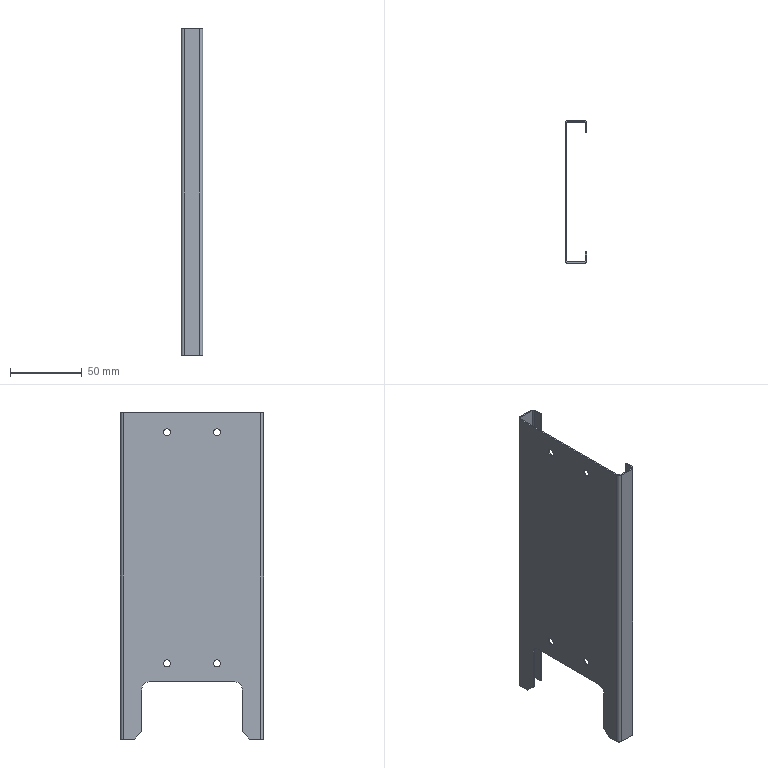Part | SolidWorks | features BaseBody 1 | 1 solid | 54 faces | box 15 x 100 x 228 mm | volume 28896 mm3 | plane 36 | cylinder 18 | commonest cylinder face diameters 5 x8 2 x4 4 x4 10 x2
STEP:
#1=CARTESIAN_POINT('',(0.,90.,-114.));
#2=VERTEX_POINT('',#1);
#3=CARTESIAN_POINT('',(0.,85.,-109.));
#4=VERTEX_POINT('',#3);
#5=CARTESIAN_POINT('',(0.,45.,-69.));
#6=DIRECTION('',(0.,-0.7071,0.7071));
#7=VECTOR('',#6,1000.);
#8=LINE('',#5,#7);
#9=EDGE_CURVE('',#2,#4,#8,.T.);
#10=ORIENTED_EDGE('',*,*,#9,.F.);
#11=CARTESIAN_POINT('',(1.,90.,-114.));
#12=VERTEX_POINT('',#11);
#13=CARTESIAN_POINT('',(0.,90.,-114.));
#14=DIRECTION('',(-1.,0.,0.));
#15=VECTOR('',#14,1000.);
#16=LINE('',#13,#15);
#17=EDGE_CURVE('',#12,#2,#16,.T.);
#18=ORIENTED_EDGE('',*,*,#17,.F.);
#19=CARTESIAN_POINT('',(1.,85.,-109.));
#20=VERTEX_POINT('',#19);
#21=CARTESIAN_POINT('',(1.,85.,-109.));
#22=DIRECTION('',(0.,0.7071,-0.7071));
#23=VECTOR('',#22,1000.);
#24=LINE('',#21,#23);
#25=EDGE_CURVE('',#20,#12,#24,.T.);
#26=ORIENTED_EDGE('',*,*,#25,.F.);
#27=CARTESIAN_POINT('',(1.,85.,-109.));
#28=DIRECTION('',(1.,0.,0.));
#29=VECTOR('',#28,1000.);
#30=LINE('',#27,#29);
#31=EDGE_CURVE('',#4,#20,#30,.T.);
#32=ORIENTED_EDGE('',*,*,#31,.F.);
#33=EDGE_LOOP('',(#10,#18,#26,#32));
#34=FACE_OUTER_BOUND('',#33,.T.);
#35=CARTESIAN_POINT('',(10.,85.,-109.));
#36=DIRECTION('',(0.,-0.7071,-0.7071));
#37=DIRECTION('',(0.,-0.7071,0.7071));
#38=AXIS2_PLACEMENT_3D('',#35,#36,#37);
#39=PLANE('',#38);
#40=ADVANCED_FACE('',(#34),#39,.T.);
#41=CARTESIAN_POINT('',(1.,10.,-114.));
#42=VERTEX_POINT('',#41);
#43=CARTESIAN_POINT('',(1.,15.,-109.));
#44=VERTEX_POINT('',#43);
#45=CARTESIAN_POINT('',(1.,15.,-109.));
#46=DIRECTION('',(0.,0.7071,0.7071));
#47=VECTOR('',#46,1000.);
#48=LINE('',#45,#47);
#49=EDGE_CURVE('',#42,#44,#48,.T.);
#50=ORIENTED_EDGE('',*,*,#49,.F.);
#51=CARTESIAN_POINT('',(0.,10.,-114.));
#52=VERTEX_POINT('',#51);
#53=CARTESIAN_POINT('',(1.,10.,-114.));
#54=DIRECTION('',(1.,0.,0.));
#55=VECTOR('',#54,1000.);
#56=LINE('',#53,#55);
#57=EDGE_CURVE('',#52,#42,#56,.T.);
#58=ORIENTED_EDGE('',*,*,#57,.F.);
#59=CARTESIAN_POINT('',(0.,15.,-109.));
#60=VERTEX_POINT('',#59);
#61=CARTESIAN_POINT('',(0.,5.,-119.));
#62=DIRECTION('',(0.,-0.7071,-0.7071));
#63=VECTOR('',#62,1000.);
#64=LINE('',#61,#63);
#65=EDGE_CURVE('',#60,#52,#64,.T.);
#66=ORIENTED_EDGE('',*,*,#65,.F.);
#67=CARTESIAN_POINT('',(0.,15.,-109.));
#68=DIRECTION('',(-1.,0.,0.));
#69=VECTOR('',#68,1000.);
#70=LINE('',#67,#69);
#71=EDGE_CURVE('',#44,#60,#70,.T.);
#72=ORIENTED_EDGE('',*,*,#71,.F.);
#73=EDGE_LOOP('',(#50,#58,#66,#72));
#74=FACE_OUTER_BOUND('',#73,.T.);
#75=CARTESIAN_POINT('',(10.,15.,-109.));
#76=DIRECTION('',(0.,0.7071,-0.7071));
#77=DIRECTION('',(-1.,0.,0.));
#78=AXIS2_PLACEMENT_3D('',#75,#76,#77);
#79=PLANE('',#78);
#80=ADVANCED_FACE('',(#74),#79,.T.);
#81=CARTESIAN_POINT('',(1.,80.,-74.));
#82=VERTEX_POINT('',#81);
#83=CARTESIAN_POINT('',(1.,85.,-79.));
#84=VERTEX_POINT('',#83);
#85=CARTESIAN_POINT('',(1.,80.,-79.));
#86=DIRECTION('',(-1.,0.,0.));
#87=DIRECTION('',(0.,0.,1.));
#88=AXIS2_PLACEMENT_3D('',#85,#86,#87);
#89=CIRCLE('',#88,5.);
#90=EDGE_CURVE('',#82,#84,#89,.T.);
#91=ORIENTED_EDGE('',*,*,#90,.F.);
#92=CARTESIAN_POINT('',(0.,80.,-74.));
#93=VERTEX_POINT('',#92);
#94=CARTESIAN_POINT('',(1.,80.,-74.));
#95=DIRECTION('',(1.,0.,0.));
#96=VECTOR('',#95,1000.);
#97=LINE('',#94,#96);
#98=EDGE_CURVE('',#93,#82,#97,.T.);
#99=ORIENTED_EDGE('',*,*,#98,.F.);
#100=CARTESIAN_POINT('',(0.,85.,-79.));
#101=VERTEX_POINT('',#100);
#102=CARTESIAN_POINT('',(0.,80.,-79.));
#103=DIRECTION('',(1.,0.,0.));
#104=DIRECTION('',(0.,0.,1.));
#105=AXIS2_PLACEMENT_3D('',#102,#103,#104);
#106=CIRCLE('',#105,5.);
#107=EDGE_CURVE('',#101,#93,#106,.T.);
#108=ORIENTED_EDGE('',*,*,#107,.F.);
#109=CARTESIAN_POINT('',(0.,85.,-79.));
#110=DIRECTION('',(-1.,0.,0.));
#111=VECTOR('',#110,1000.);
#112=LINE('',#109,#111);
#113=EDGE_CURVE('',#84,#101,#112,.T.);
#114=ORIENTED_EDGE('',*,*,#113,.F.);
#115=EDGE_LOOP('',(#91,#99,#108,#114));
#116=FACE_OUTER_BOUND('',#115,.T.);
#117=CARTESIAN_POINT('',(10.,80.,-79.));
#118=DIRECTION('',(1.,0.,0.));
#119=DIRECTION('',(0.,0.,-1.));
#120=AXIS2_PLACEMENT_3D('',#117,#118,#119);
#121=CYLINDRICAL_SURFACE('',#120,5.);
#122=ADVANCED_FACE('',(#116),#121,.F.);
#123=CARTESIAN_POINT('',(1.,15.,-79.));
#124=VERTEX_POINT('',#123);
#125=CARTESIAN_POINT('',(1.,20.,-74.));
#126=VERTEX_POINT('',#125);
#127=CARTESIAN_POINT('',(1.,20.,-79.));
#128=DIRECTION('',(-1.,0.,0.));
#129=DIRECTION('',(0.,0.,1.));
#130=AXIS2_PLACEMENT_3D('',#127,#128,#129);
#131=CIRCLE('',#130,5.);
#132=EDGE_CURVE('',#124,#126,#131,.T.);
#133=ORIENTED_EDGE('',*,*,#132,.F.);
#134=CARTESIAN_POINT('',(0.,15.,-79.));
#135=VERTEX_POINT('',#134);
#136=CARTESIAN_POINT('',(1.,15.,-79.));
#137=DIRECTION('',(1.,0.,0.));
#138=VECTOR('',#137,1000.);
#139=LINE('',#136,#138);
#140=EDGE_CURVE('',#135,#124,#139,.T.);
#141=ORIENTED_EDGE('',*,*,#140,.F.);
#142=CARTESIAN_POINT('',(0.,20.,-74.));
#143=VERTEX_POINT('',#142);
#144=CARTESIAN_POINT('',(0.,20.,-79.));
#145=DIRECTION('',(1.,0.,0.));
#146=DIRECTION('',(0.,0.,1.));
#147=AXIS2_PLACEMENT_3D('',#144,#145,#146);
#148=CIRCLE('',#147,5.);
#149=EDGE_CURVE('',#143,#135,#148,.T.);
#150=ORIENTED_EDGE('',*,*,#149,.F.);
#151=CARTESIAN_POINT('',(0.,20.,-74.));
#152=DIRECTION('',(-1.,0.,0.));
#153=VECTOR('',#152,1000.);
#154=LINE('',#151,#153);
#155=EDGE_CURVE('',#126,#143,#154,.T.);
#156=ORIENTED_EDGE('',*,*,#155,.F.);
#157=EDGE_LOOP('',(#133,#141,#150,#156));
#158=FACE_OUTER_BOUND('',#157,.T.);
#159=CARTESIAN_POINT('',(10.,20.,-79.));
#160=DIRECTION('',(1.,0.,0.));
#161=DIRECTION('',(0.,0.,-1.));
#162=AXIS2_PLACEMENT_3D('',#159,#160,#161);
#163=CYLINDRICAL_SURFACE('',#162,5.);
#164=ADVANCED_FACE('',(#158),#163,.F.);
#165=CARTESIAN_POINT('',(1.,67.5,98.));
#166=VERTEX_POINT('',#165);
#167=CARTESIAN_POINT('',(0.,67.5,98.));
#168=VERTEX_POINT('',#167);
#169=CARTESIAN_POINT('',(10.,67.5,98.));
#170=DIRECTION('',(-1.,0.,0.));
#171=VECTOR('',#170,1000.);
#172=LINE('',#169,#171);
#173=EDGE_CURVE('',#166,#168,#172,.T.);
#174=ORIENTED_EDGE('',*,*,#173,.F.);
#175=CARTESIAN_POINT('',(1.,67.5,103.));
#176=VERTEX_POINT('',#175);
#177=CARTESIAN_POINT('',(1.,67.5,100.5));
#178=DIRECTION('',(-1.,0.,0.));
#179=DIRECTION('',(0.,0.,1.));
#180=AXIS2_PLACEMENT_3D('',#177,#178,#179);
#181=CIRCLE('',#180,2.5);
#182=EDGE_CURVE('',#176,#166,#181,.T.);
#183=ORIENTED_EDGE('',*,*,#182,.F.);
#184=CARTESIAN_POINT('',(0.,67.5,103.));
#185=VERTEX_POINT('',#184);
#186=CARTESIAN_POINT('',(10.,67.5,103.));
#187=DIRECTION('',(-1.,0.,0.));
#188=VECTOR('',#187,1000.);
#189=LINE('',#186,#188);
#190=EDGE_CURVE('',#176,#185,#189,.T.);
#191=ORIENTED_EDGE('',*,*,#190,.T.);
#192=CARTESIAN_POINT('',(0.,67.5,100.5));
#193=DIRECTION('',(-1.,0.,0.));
#194=DIRECTION('',(0.,0.,1.));
#195=AXIS2_PLACEMENT_3D('',#192,#193,#194);
#196=CIRCLE('',#195,2.5);
#197=EDGE_CURVE('',#185,#168,#196,.T.);
#198=ORIENTED_EDGE('',*,*,#197,.T.);
#199=EDGE_LOOP('',(#174,#183,#191,#198));
#200=FACE_OUTER_BOUND('',#199,.T.);
#201=CARTESIAN_POINT('',(10.,67.5,100.5));
#202=DIRECTION('',(-1.,0.,0.));
#203=DIRECTION('',(0.,0.,1.));
#204=AXIS2_PLACEMENT_3D('',#201,#202,#203);
#205=CYLINDRICAL_SURFACE('',#204,2.5);
#206=ADVANCED_FACE('',(#200),#205,.F.);
#207=CARTESIAN_POINT('',(1.,32.5,-63.6));
#208=VERTEX_POINT('',#207);
#209=CARTESIAN_POINT('',(0.,32.5,-63.6));
#210=VERTEX_POINT('',#209);
#211=CARTESIAN_POINT('',(10.,32.5,-63.6));
#212=DIRECTION('',(-1.,0.,0.));
#213=VECTOR('',#212,1000.);
#214=LINE('',#211,#213);
#215=EDGE_CURVE('',#208,#210,#214,.T.);
#216=ORIENTED_EDGE('',*,*,#215,.F.);
#217=CARTESIAN_POINT('',(1.,32.5,-58.6));
#218=VERTEX_POINT('',#217);
#219=CARTESIAN_POINT('',(1.,32.5,-61.1));
#220=DIRECTION('',(-1.,0.,0.));
#221=DIRECTION('',(0.,0.,1.));
#222=AXIS2_PLACEMENT_3D('',#219,#220,#221);
#223=CIRCLE('',#222,2.5);
#224=EDGE_CURVE('',#218,#208,#223,.T.);
#225=ORIENTED_EDGE('',*,*,#224,.F.);
#226=CARTESIAN_POINT('',(0.,32.5,-58.6));
#227=VERTEX_POINT('',#226);
#228=CARTESIAN_POINT('',(10.,32.5,-58.6));
#229=DIRECTION('',(-1.,0.,0.));
#230=VECTOR('',#229,1000.);
#231=LINE('',#228,#230);
#232=EDGE_CURVE('',#218,#227,#231,.T.);
#233=ORIENTED_EDGE('',*,*,#232,.T.);
#234=CARTESIAN_POINT('',(0.,32.5,-61.1));
#235=DIRECTION('',(-1.,0.,0.));
#236=DIRECTION('',(0.,0.,1.));
#237=AXIS2_PLACEMENT_3D('',#234,#235,#236);
#238=CIRCLE('',#237,2.5);
#239=EDGE_CURVE('',#227,#210,#238,.T.);
#240=ORIENTED_EDGE('',*,*,#239,.T.);
#241=EDGE_LOOP('',(#216,#225,#233,#240));
#242=FACE_OUTER_BOUND('',#241,.T.);
#243=CARTESIAN_POINT('',(10.,32.5,-61.1));
#244=DIRECTION('',(-1.,0.,0.));
#245=DIRECTION('',(0.,0.,1.));
#246=AXIS2_PLACEMENT_3D('',#243,#244,#245);
#247=CYLINDRICAL_SURFACE('',#246,2.5);
#248=ADVANCED_FACE('',(#242),#247,.F.);
#249=CARTESIAN_POINT('',(1.,67.5,-63.6));
#250=VERTEX_POINT('',#249);
#251=CARTESIAN_POINT('',(0.,67.5,-63.6));
#252=VERTEX_POINT('',#251);
#253=CARTESIAN_POINT('',(10.,67.5,-63.6));
#254=DIRECTION('',(-1.,0.,0.));
#255=VECTOR('',#254,1000.);
#256=LINE('',#253,#255);
#257=EDGE_CURVE('',#250,#252,#256,.T.);
#258=ORIENTED_EDGE('',*,*,#257,.F.);
#259=CARTESIAN_POINT('',(1.,67.5,-58.6));
#260=VERTEX_POINT('',#259);
#261=CARTESIAN_POINT('',(1.,67.5,-61.1));
#262=DIRECTION('',(-1.,0.,0.));
#263=DIRECTION('',(0.,0.,1.));
#264=AXIS2_PLACEMENT_3D('',#261,#262,#263);
#265=CIRCLE('',#264,2.5);
#266=EDGE_CURVE('',#260,#250,#265,.T.);
#267=ORIENTED_EDGE('',*,*,#266,.F.);
#268=CARTESIAN_POINT('',(0.,67.5,-58.6));
#269=VERTEX_POINT('',#268);
#270=CARTESIAN_POINT('',(10.,67.5,-58.6));
#271=DIRECTION('',(-1.,0.,0.));
#272=VECTOR('',#271,1000.);
#273=LINE('',#270,#272);
#274=EDGE_CURVE('',#260,#269,#273,.T.);
#275=ORIENTED_EDGE('',*,*,#274,.T.);
#276=CARTESIAN_POINT('',(0.,67.5,-61.1));
#277=DIRECTION('',(-1.,0.,0.));
#278=DIRECTION('',(0.,0.,1.));
#279=AXIS2_PLACEMENT_3D('',#276,#277,#278);
#280=CIRCLE('',#279,2.5);
#281=EDGE_CURVE('',#269,#252,#280,.T.);
#282=ORIENTED_EDGE('',*,*,#281,.T.);
#283=EDGE_LOOP('',(#258,#267,#275,#282));
#284=FACE_OUTER_BOUND('',#283,.T.);
#285=CARTESIAN_POINT('',(10.,67.5,-61.1));
#286=DIRECTION('',(-1.,0.,0.));
#287=DIRECTION('',(0.,0.,1.));
#288=AXIS2_PLACEMENT_3D('',#285,#286,#287);
#289=CYLINDRICAL_SURFACE('',#288,2.5);
#290=ADVANCED_FACE('',(#284),#289,.F.);
#291=CARTESIAN_POINT('',(0.,85.,-154.));
#292=DIRECTION('',(0.,0.,-1.));
#293=VECTOR('',#292,1000.);
#294=LINE('',#291,#293);
#295=EDGE_CURVE('',#101,#4,#294,.T.);
#296=ORIENTED_EDGE('',*,*,#295,.T.);
#297=ORIENTED_EDGE('',*,*,#31,.T.);
#298=CARTESIAN_POINT('',(1.,85.,-114.));
#299=DIRECTION('',(0.,0.,-1.));
#300=VECTOR('',#299,1000.);
#301=LINE('',#298,#300);
#302=EDGE_CURVE('',#84,#20,#301,.T.);
#303=ORIENTED_EDGE('',*,*,#302,.F.);
#304=ORIENTED_EDGE('',*,*,#113,.T.);
#305=EDGE_LOOP('',(#296,#297,#303,#304));
#306=FACE_OUTER_BOUND('',#305,.T.);
#307=CARTESIAN_POINT('',(10.,85.,-154.));
#308=DIRECTION('',(0.,1.,0.));
#309=DIRECTION('',(1.,0.,0.));
#310=AXIS2_PLACEMENT_3D('',#307,#308,#309);
#311=PLANE('',#310);
#312=ADVANCED_FACE('',(#306),#311,.F.);
#313=CARTESIAN_POINT('',(1.,15.,-114.));
#314=DIRECTION('',(0.,0.,1.));
#315=VECTOR('',#314,1000.);
#316=LINE('',#313,#315);
#317=EDGE_CURVE('',#44,#124,#316,.T.);
#318=ORIENTED_EDGE('',*,*,#317,.F.);
#319=ORIENTED_EDGE('',*,*,#71,.T.);
#320=CARTESIAN_POINT('',(0.,15.,-154.));
#321=DIRECTION('',(0.,0.,1.));
#322=VECTOR('',#321,1000.);
#323=LINE('',#320,#322);
#324=EDGE_CURVE('',#60,#135,#323,.T.);
#325=ORIENTED_EDGE('',*,*,#324,.T.);
#326=ORIENTED_EDGE('',*,*,#140,.T.);
#327=EDGE_LOOP('',(#318,#319,#325,#326));
#328=FACE_OUTER_BOUND('',#327,.T.);
#329=CARTESIAN_POINT('',(10.,15.,-154.));
#330=DIRECTION('',(0.,-1.,0.));
#331=DIRECTION('',(0.,0.,-1.));
#332=AXIS2_PLACEMENT_3D('',#329,#330,#331);
#333=PLANE('',#332);
#334=ADVANCED_FACE('',(#328),#333,.F.);
#335=CARTESIAN_POINT('',(1.,0.,-74.));
#336=DIRECTION('',(0.,1.,0.));
#337=VECTOR('',#336,1000.);
#338=LINE('',#335,#337);
#339=EDGE_CURVE('',#126,#82,#338,.T.);
#340=ORIENTED_EDGE('',*,*,#339,.F.);
#341=ORIENTED_EDGE('',*,*,#155,.T.);
#342=CARTESIAN_POINT('',(0.,15.,-74.));
#343=DIRECTION('',(0.,1.,0.));
#344=VECTOR('',#343,1000.);
#345=LINE('',#342,#344);
#346=EDGE_CURVE('',#143,#93,#345,.T.);
#347=ORIENTED_EDGE('',*,*,#346,.T.);
#348=ORIENTED_EDGE('',*,*,#98,.T.);
#349=EDGE_LOOP('',(#340,#341,#347,#348));
#350=FACE_OUTER_BOUND('',#349,.T.);
#351=CARTESIAN_POINT('',(10.,15.,-74.));
#352=DIRECTION('',(0.,0.,1.));
#353=DIRECTION('',(1.,0.,0.));
#354=AXIS2_PLACEMENT_3D('',#351,#352,#353);
#355=PLANE('',#354);
#356=ADVANCED_FACE('',(#350),#355,.F.);
#357=CARTESIAN_POINT('',(1.,32.5,98.));
#358=VERTEX_POINT('',#357);
#359=CARTESIAN_POINT('',(0.,32.5,98.));
#360=VERTEX_POINT('',#359);
#361=CARTESIAN_POINT('',(10.,32.5,98.));
#362=DIRECTION('',(-1.,0.,0.));
#363=VECTOR('',#362,1000.);
#364=LINE('',#361,#363);
#365=EDGE_CURVE('',#358,#360,#364,.T.);
#366=ORIENTED_EDGE('',*,*,#365,.F.);
#367=CARTESIAN_POINT('',(1.,32.5,103.));
#368=VERTEX_POINT('',#367);
#369=CARTESIAN_POINT('',(1.,32.5,100.5));
#370=DIRECTION('',(-1.,0.,0.));
#371=DIRECTION('',(0.,0.,1.));
#372=AXIS2_PLACEMENT_3D('',#369,#370,#371);
#373=CIRCLE('',#372,2.5);
#374=EDGE_CURVE('',#368,#358,#373,.T.);
#375=ORIENTED_EDGE('',*,*,#374,.F.);
#376=CARTESIAN_POINT('',(0.,32.5,103.));
#377=VERTEX_POINT('',#376);
#378=CARTESIAN_POINT('',(10.,32.5,103.));
#379=DIRECTION('',(-1.,0.,0.));
#380=VECTOR('',#379,1000.);
#381=LINE('',#378,#380);
#382=EDGE_CURVE('',#368,#377,#381,.T.);
#383=ORIENTED_EDGE('',*,*,#382,.T.);
#384=CARTESIAN_POINT('',(0.,32.5,100.5));
#385=DIRECTION('',(-1.,0.,0.));
#386=DIRECTION('',(0.,0.,1.));
#387=AXIS2_PLACEMENT_3D('',#384,#385,#386);
#388=CIRCLE('',#387,2.5);
#389=EDGE_CURVE('',#377,#360,#388,.T.);
#390=ORIENTED_EDGE('',*,*,#389,.T.);
#391=EDGE_LOOP('',(#366,#375,#383,#390));
#392=FACE_OUTER_BOUND('',#391,.T.);
#393=CARTESIAN_POINT('',(10.,32.5,100.5));
#394=DIRECTION('',(-1.,0.,0.));
#395=DIRECTION('',(0.,0.,1.));
#396=AXIS2_PLACEMENT_3D('',#393,#394,#395);
#397=CYLINDRICAL_SURFACE('',#396,2.5);
#398=ADVANCED_FACE('',(#392),#397,.F.);
#399=CARTESIAN_POINT('',(15.,2.,114.));
#400=VERTEX_POINT('',#399);
#401=CARTESIAN_POINT('',(15.,8.,114.));
#402=VERTEX_POINT('',#401);
#403=CARTESIAN_POINT('',(15.,0.,114.));
#404=DIRECTION('',(0.,1.,0.));
#405=VECTOR('',#404,1000.);
#406=LINE('',#403,#405);
#407=EDGE_CURVE('',#400,#402,#406,.T.);
#408=ORIENTED_EDGE('',*,*,#407,.T.);
#409=CARTESIAN_POINT('',(14.,8.,114.));
#410=VERTEX_POINT('',#409);
#411=CARTESIAN_POINT('',(14.,8.,114.));
#412=DIRECTION('',(1.,0.,0.));
#413=VECTOR('',#412,1000.);
#414=LINE('',#411,#413);
#415=EDGE_CURVE('',#410,#402,#414,.T.);
#416=ORIENTED_EDGE('',*,*,#415,.F.);
#417=CARTESIAN_POINT('',(14.,2.,114.));
#418=VERTEX_POINT('',#417);
#419=CARTESIAN_POINT('',(14.,0.,114.));
#420=DIRECTION('',(0.,1.,0.));
#421=VECTOR('',#420,1000.);
#422=LINE('',#419,#421);
#423=EDGE_CURVE('',#418,#410,#422,.T.);
#424=ORIENTED_EDGE('',*,*,#423,.F.);
#425=CARTESIAN_POINT('',(14.,2.,114.));
#426=DIRECTION('',(1.,0.,0.));
#427=VECTOR('',#426,1000.);
#428=LINE('',#425,#427);
#429=EDGE_CURVE('',#418,#400,#428,.T.);
#430=ORIENTED_EDGE('',*,*,#429,.T.);
#431=EDGE_LOOP('',(#408,#416,#424,#430));
#432=FACE_OUTER_BOUND('',#431,.T.);
#433=CARTESIAN_POINT('',(13.,2.,114.));
#434=DIRECTION('',(0.,0.,1.));
#435=DIRECTION('',(1.,0.,0.));
#436=AXIS2_PLACEMENT_3D('',#433,#434,#435);
#437=PLANE('',#436);
#438=ADVANCED_FACE('',(#432),#437,.T.);
#439=CARTESIAN_POINT('',(14.,92.,-114.));
#440=VERTEX_POINT('',#439);
#441=CARTESIAN_POINT('',(14.,98.,-114.));
#442=VERTEX_POINT('',#441);
#443=CARTESIAN_POINT('',(14.,100.,-114.));
#444=DIRECTION('',(0.,1.,0.));
#445=VECTOR('',#444,1000.);
#446=LINE('',#443,#445);
#447=EDGE_CURVE('',#440,#442,#446,.T.);
#448=ORIENTED_EDGE('',*,*,#447,.T.);
#449=CARTESIAN_POINT('',(15.,98.,-114.));
#450=VERTEX_POINT('',#449);
#451=CARTESIAN_POINT('',(14.,98.,-114.));
#452=DIRECTION('',(1.,0.,0.));
#453=VECTOR('',#452,1000.);
#454=LINE('',#451,#453);
#455=EDGE_CURVE('',#442,#450,#454,.T.);
#456=ORIENTED_EDGE('',*,*,#455,.T.);
#457=CARTESIAN_POINT('',(15.,92.,-114.));
#458=VERTEX_POINT('',#457);
#459=CARTESIAN_POINT('',(15.,100.,-114.));
#460=DIRECTION('',(0.,1.,0.));
#461=VECTOR('',#460,1000.);
#462=LINE('',#459,#461);
#463=EDGE_CURVE('',#458,#450,#462,.T.);
#464=ORIENTED_EDGE('',*,*,#463,.F.);
#465=CARTESIAN_POINT('',(15.,92.,-114.));
#466=DIRECTION('',(-1.,0.,0.));
#467=VECTOR('',#466,1000.);
#468=LINE('',#465,#467);
#469=EDGE_CURVE('',#458,#440,#468,.T.);
#470=ORIENTED_EDGE('',*,*,#469,.T.);
#471=EDGE_LOOP('',(#448,#456,#464,#470));
#472=FACE_OUTER_BOUND('',#471,.T.);
#473=CARTESIAN_POINT('',(13.,2.,-114.));
#474=DIRECTION('',(0.,0.,1.));
#475=DIRECTION('',(1.,0.,0.));
#476=AXIS2_PLACEMENT_3D('',#473,#474,#475);
#477=PLANE('',#476);
#478=ADVANCED_FACE('',(#472),#477,.F.);
#479=ORIENTED_EDGE('',*,*,#415,.T.);
#480=CARTESIAN_POINT('',(15.,8.,-114.));
#481=VERTEX_POINT('',#480);
#482=CARTESIAN_POINT('',(15.,8.,-114.));
#483=DIRECTION('',(0.,0.,1.));
#484=VECTOR('',#483,1000.);
#485=LINE('',#482,#484);
#486=EDGE_CURVE('',#481,#402,#485,.T.);
#487=ORIENTED_EDGE('',*,*,#486,.F.);
#488=CARTESIAN_POINT('',(14.,8.,-114.));
#489=VERTEX_POINT('',#488);
#490=CARTESIAN_POINT('',(14.,8.,-114.));
#491=DIRECTION('',(1.,0.,0.));
#492=VECTOR('',#491,1000.);
#493=LINE('',#490,#492);
#494=EDGE_CURVE('',#489,#481,#493,.T.);
#495=ORIENTED_EDGE('',*,*,#494,.F.);
#496=CARTESIAN_POINT('',(14.,8.,-114.));
#497=DIRECTION('',(0.,0.,1.));
#498=VECTOR('',#497,1000.);
#499=LINE('',#496,#498);
#500=EDGE_CURVE('',#489,#410,#499,.T.);
#501=ORIENTED_EDGE('',*,*,#500,.T.);
#502=EDGE_LOOP('',(#479,#487,#495,#501));
#503=FACE_OUTER_BOUND('',#502,.T.);
#504=CARTESIAN_POINT('',(14.,8.,-114.));
#505=DIRECTION('',(0.,-1.,0.));
#506=DIRECTION('',(0.,0.,-1.));
#507=AXIS2_PLACEMENT_3D('',#504,#505,#506);
#508=PLANE('',#507);
#509=ADVANCED_FACE('',(#503),#508,.F.);
#510=ORIENTED_EDGE('',*,*,#423,.T.);
#511=ORIENTED_EDGE('',*,*,#500,.F.);
#512=CARTESIAN_POINT('',(14.,2.,-114.));
#513=VERTEX_POINT('',#512);
#514=CARTESIAN_POINT('',(14.,0.,-114.));
#515=DIRECTION('',(0.,1.,0.));
#516=VECTOR('',#515,1000.);
#517=LINE('',#514,#516);
#518=EDGE_CURVE('',#513,#489,#517,.T.);
#519=ORIENTED_EDGE('',*,*,#518,.F.);
#520=CARTESIAN_POINT('',(14.,2.,-114.));
#521=DIRECTION('',(0.,0.,1.));
#522=VECTOR('',#521,1000.);
#523=LINE('',#520,#522);
#524=EDGE_CURVE('',#513,#418,#523,.T.);
#525=ORIENTED_EDGE('',*,*,#524,.T.);
#526=EDGE_LOOP('',(#510,#511,#519,#525));
#527=FACE_OUTER_BOUND('',#526,.T.);
#528=CARTESIAN_POINT('',(14.,0.,-114.));
#529=DIRECTION('',(1.,0.,0.));
#530=DIRECTION('',(0.,1.,0.));
#531=AXIS2_PLACEMENT_3D('',#528,#529,#530);
#532=PLANE('',#531);
#533=ADVANCED_FACE('',(#527),#532,.F.);
#534=CARTESIAN_POINT('',(13.,1.,114.));
#535=VERTEX_POINT('',#534);
#536=CARTESIAN_POINT('',(13.,2.,114.));
#537=DIRECTION('',(0.,0.,1.));
#538=DIRECTION('',(1.,0.,0.));
#539=AXIS2_PLACEMENT_3D('',#536,#537,#538);
#540=CIRCLE('',#539,1.);
#541=EDGE_CURVE('',#535,#418,#540,.T.);
#542=ORIENTED_EDGE('',*,*,#541,.T.);
#543=ORIENTED_EDGE('',*,*,#524,.F.);
#544=CARTESIAN_POINT('',(13.,1.,-114.));
#545=VERTEX_POINT('',#544);
#546=CARTESIAN_POINT('',(13.,2.,-114.));
#547=DIRECTION('',(0.,0.,1.));
#548=DIRECTION('',(1.,0.,0.));
#549=AXIS2_PLACEMENT_3D('',#546,#547,#548);
#550=CIRCLE('',#549,1.);
#551=EDGE_CURVE('',#545,#513,#550,.T.);
#552=ORIENTED_EDGE('',*,*,#551,.F.);
#553=CARTESIAN_POINT('',(13.,1.,-114.));
#554=DIRECTION('',(0.,0.,1.));
#555=VECTOR('',#554,1000.);
#556=LINE('',#553,#555);
#557=EDGE_CURVE('',#545,#535,#556,.T.);
#558=ORIENTED_EDGE('',*,*,#557,.T.);
#559=EDGE_LOOP('',(#542,#543,#552,#558));
#560=FACE_OUTER_BOUND('',#559,.T.);
#561=CARTESIAN_POINT('',(13.,2.,-114.));
#562=DIRECTION('',(0.,0.,1.));
#563=DIRECTION('',(1.,0.,0.));
#564=AXIS2_PLACEMENT_3D('',#561,#562,#563);
#565=CYLINDRICAL_SURFACE('',#564,1.);
#566=ADVANCED_FACE('',(#560),#565,.F.);
#567=CARTESIAN_POINT('',(2.,1.,114.));
#568=VERTEX_POINT('',#567);
#569=CARTESIAN_POINT('',(0.,1.,114.));
#570=DIRECTION('',(1.,0.,0.));
#571=VECTOR('',#570,1000.);
#572=LINE('',#569,#571);
#573=EDGE_CURVE('',#568,#535,#572,.T.);
#574=ORIENTED_EDGE('',*,*,#573,.T.);
#575=ORIENTED_EDGE('',*,*,#557,.F.);
#576=CARTESIAN_POINT('',(2.,1.,-114.));
#577=VERTEX_POINT('',#576);
#578=CARTESIAN_POINT('',(0.,1.,-114.));
#579=DIRECTION('',(1.,0.,0.));
#580=VECTOR('',#579,1000.);
#581=LINE('',#578,#580);
#582=EDGE_CURVE('',#577,#545,#581,.T.);
#583=ORIENTED_EDGE('',*,*,#582,.F.);
#584=CARTESIAN_POINT('',(2.,1.,-114.));
#585=DIRECTION('',(0.,0.,1.));
#586=VECTOR('',#585,1000.);
#587=LINE('',#584,#586);
#588=EDGE_CURVE('',#577,#568,#587,.T.);
#589=ORIENTED_EDGE('',*,*,#588,.T.);
#590=EDGE_LOOP('',(#574,#575,#583,#589));
#591=FACE_OUTER_BOUND('',#590,.T.);
#592=CARTESIAN_POINT('',(0.,1.,-114.));
#593=DIRECTION('',(0.,-1.,0.));
#594=DIRECTION('',(0.,0.,-1.));
#595=AXIS2_PLACEMENT_3D('',#592,#593,#594);
#596=PLANE('',#595);
#597=ADVANCED_FACE('',(#591),#596,.F.);
#598=CARTESIAN_POINT('',(1.,2.,114.));
#599=VERTEX_POINT('',#598);
#600=CARTESIAN_POINT('',(2.,2.,114.));
#601=DIRECTION('',(0.,0.,1.));
#602=DIRECTION('',(1.,0.,0.));
#603=AXIS2_PLACEMENT_3D('',#600,#601,#602);
#604=CIRCLE('',#603,1.);
#605=EDGE_CURVE('',#599,#568,#604,.T.);
#606=ORIENTED_EDGE('',*,*,#605,.T.);
#607=ORIENTED_EDGE('',*,*,#588,.F.);
#608=CARTESIAN_POINT('',(1.,2.,-114.));
#609=VERTEX_POINT('',#608);
#610=CARTESIAN_POINT('',(2.,2.,-114.));
#611=DIRECTION('',(0.,0.,1.));
#612=DIRECTION('',(1.,0.,0.));
#613=AXIS2_PLACEMENT_3D('',#610,#611,#612);
#614=CIRCLE('',#613,1.);
#615=EDGE_CURVE('',#609,#577,#614,.T.);
#616=ORIENTED_EDGE('',*,*,#615,.F.);
#617=CARTESIAN_POINT('',(1.,2.,-114.));
#618=DIRECTION('',(0.,0.,1.));
#619=VECTOR('',#618,1000.);
#620=LINE('',#617,#619);
#621=EDGE_CURVE('',#609,#599,#620,.T.);
#622=ORIENTED_EDGE('',*,*,#621,.T.);
#623=EDGE_LOOP('',(#606,#607,#616,#622));
#624=FACE_OUTER_BOUND('',#623,.T.);
#625=CARTESIAN_POINT('',(2.,2.,-114.));
#626=DIRECTION('',(0.,0.,1.));
#627=DIRECTION('',(1.,0.,0.));
#628=AXIS2_PLACEMENT_3D('',#625,#626,#627);
#629=CYLINDRICAL_SURFACE('',#628,1.);
#630=ADVANCED_FACE('',(#624),#629,.F.);
#631=ORIENTED_EDGE('',*,*,#374,.T.);
#632=CARTESIAN_POINT('',(1.,32.5,100.5));
#633=DIRECTION('',(-1.,0.,0.));
#634=DIRECTION('',(0.,0.,1.));
#635=AXIS2_PLACEMENT_3D('',#632,#633,#634);
#636=CIRCLE('',#635,2.5);
#637=EDGE_CURVE('',#358,#368,#636,.T.);
#638=ORIENTED_EDGE('',*,*,#637,.T.);
#639=EDGE_LOOP('',(#631,#638));
#640=FACE_BOUND('',#639,.T.);
#641=ORIENTED_EDGE('',*,*,#266,.T.);
#642=CARTESIAN_POINT('',(1.,67.5,-61.1));
#643=DIRECTION('',(-1.,0.,0.));
#644=DIRECTION('',(0.,0.,1.));
#645=AXIS2_PLACEMENT_3D('',#642,#643,#644);
#646=CIRCLE('',#645,2.5);
#647=EDGE_CURVE('',#250,#260,#646,.T.);
#648=ORIENTED_EDGE('',*,*,#647,.T.);
#649=EDGE_LOOP('',(#641,#648));
#650=FACE_BOUND('',#649,.T.);
#651=ORIENTED_EDGE('',*,*,#224,.T.);
#652=CARTESIAN_POINT('',(1.,32.5,-61.1));
#653=DIRECTION('',(-1.,0.,0.));
#654=DIRECTION('',(0.,0.,1.));
#655=AXIS2_PLACEMENT_3D('',#652,#653,#654);
#656=CIRCLE('',#655,2.5);
#657=EDGE_CURVE('',#208,#218,#656,.T.);
#658=ORIENTED_EDGE('',*,*,#657,.T.);
#659=EDGE_LOOP('',(#651,#658));
#660=FACE_BOUND('',#659,.T.);
#661=ORIENTED_EDGE('',*,*,#182,.T.);
#662=CARTESIAN_POINT('',(1.,67.5,100.5));
#663=DIRECTION('',(-1.,0.,0.));
#664=DIRECTION('',(0.,0.,1.));
#665=AXIS2_PLACEMENT_3D('',#662,#663,#664);
#666=CIRCLE('',#665,2.5);
#667=EDGE_CURVE('',#166,#176,#666,.T.);
#668=ORIENTED_EDGE('',*,*,#667,.T.);
#669=EDGE_LOOP('',(#661,#668));
#670=FACE_BOUND('',#669,.T.);
#671=CARTESIAN_POINT('',(1.,0.,-114.));
#672=DIRECTION('',(0.,-1.,0.));
#673=VECTOR('',#672,1000.);
#674=LINE('',#671,#673);
#675=EDGE_CURVE('',#42,#609,#674,.T.);
#676=ORIENTED_EDGE('',*,*,#675,.F.);
#677=ORIENTED_EDGE('',*,*,#49,.T.);
#678=ORIENTED_EDGE('',*,*,#317,.T.);
#679=ORIENTED_EDGE('',*,*,#132,.T.);
#680=ORIENTED_EDGE('',*,*,#339,.T.);
#681=ORIENTED_EDGE('',*,*,#90,.T.);
#682=ORIENTED_EDGE('',*,*,#302,.T.);
#683=ORIENTED_EDGE('',*,*,#25,.T.);
#684=CARTESIAN_POINT('',(1.,98.,-114.));
#685=VERTEX_POINT('',#684);
#686=CARTESIAN_POINT('',(1.,0.,-114.));
#687=DIRECTION('',(0.,-1.,0.));
#688=VECTOR('',#687,1000.);
#689=LINE('',#686,#688);
#690=EDGE_CURVE('',#685,#12,#689,.T.);
#691=ORIENTED_EDGE('',*,*,#690,.F.);
#692=CARTESIAN_POINT('',(1.,98.,114.));
#693=VERTEX_POINT('',#692);
#694=CARTESIAN_POINT('',(1.,98.,-114.));
#695=DIRECTION('',(0.,0.,1.));
#696=VECTOR('',#695,1000.);
#697=LINE('',#694,#696);
#698=EDGE_CURVE('',#685,#693,#697,.T.);
#699=ORIENTED_EDGE('',*,*,#698,.T.);
#700=CARTESIAN_POINT('',(1.,0.,114.));
#701=DIRECTION('',(0.,-1.,0.));
#702=VECTOR('',#701,1000.);
#703=LINE('',#700,#702);
#704=EDGE_CURVE('',#693,#599,#703,.T.);
#705=ORIENTED_EDGE('',*,*,#704,.T.);
#706=ORIENTED_EDGE('',*,*,#621,.F.);
#707=EDGE_LOOP('',(#676,#677,#678,#679,#680,#681,#682,#683,#691,#699,#705,#706));
#708=FACE_OUTER_BOUND('',#707,.T.);
#709=CARTESIAN_POINT('',(1.,0.,-114.));
#710=DIRECTION('',(-1.,0.,0.));
#711=DIRECTION('',(0.,0.,1.));
#712=AXIS2_PLACEMENT_3D('',#709,#710,#711);
#713=PLANE('',#712);
#714=ADVANCED_FACE('',(#640,#650,#660,#670,#708),#713,.F.);
#715=CARTESIAN_POINT('',(2.,99.,114.));
#716=VERTEX_POINT('',#715);
#717=CARTESIAN_POINT('',(2.,98.,114.));
#718=DIRECTION('',(0.,0.,1.));
#719=DIRECTION('',(1.,0.,0.));
#720=AXIS2_PLACEMENT_3D('',#717,#718,#719);
#721=CIRCLE('',#720,1.);
#722=EDGE_CURVE('',#716,#693,#721,.T.);
#723=ORIENTED_EDGE('',*,*,#722,.T.);
#724=ORIENTED_EDGE('',*,*,#698,.F.);
#725=CARTESIAN_POINT('',(2.,99.,-114.));
#726=VERTEX_POINT('',#725);
#727=CARTESIAN_POINT('',(2.,98.,-114.));
#728=DIRECTION('',(0.,0.,1.));
#729=DIRECTION('',(1.,0.,0.));
#730=AXIS2_PLACEMENT_3D('',#727,#728,#729);
#731=CIRCLE('',#730,1.);
#732=EDGE_CURVE('',#726,#685,#731,.T.);
#733=ORIENTED_EDGE('',*,*,#732,.F.);
#734=CARTESIAN_POINT('',(2.,99.,-114.));
#735=DIRECTION('',(0.,0.,1.));
#736=VECTOR('',#735,1000.);
#737=LINE('',#734,#736);
#738=EDGE_CURVE('',#726,#716,#737,.T.);
#739=ORIENTED_EDGE('',*,*,#738,.T.);
#740=EDGE_LOOP('',(#723,#724,#733,#739));
#741=FACE_OUTER_BOUND('',#740,.T.);
#742=CARTESIAN_POINT('',(2.,98.,-114.));
#743=DIRECTION('',(0.,0.,1.));
#744=DIRECTION('',(1.,0.,0.));
#745=AXIS2_PLACEMENT_3D('',#742,#743,#744);
#746=CYLINDRICAL_SURFACE('',#745,1.);
#747=ADVANCED_FACE('',(#741),#746,.F.);
#748=CARTESIAN_POINT('',(13.,99.,114.));
#749=VERTEX_POINT('',#748);
#750=CARTESIAN_POINT('',(0.,99.,114.));
#751=DIRECTION('',(-1.,0.,0.));
#752=VECTOR('',#751,1000.);
#753=LINE('',#750,#752);
#754=EDGE_CURVE('',#749,#716,#753,.T.);
#755=ORIENTED_EDGE('',*,*,#754,.T.);
#756=ORIENTED_EDGE('',*,*,#738,.F.);
#757=CARTESIAN_POINT('',(13.,99.,-114.));
#758=VERTEX_POINT('',#757);
#759=CARTESIAN_POINT('',(0.,99.,-114.));
#760=DIRECTION('',(-1.,0.,0.));
#761=VECTOR('',#760,1000.);
#762=LINE('',#759,#761);
#763=EDGE_CURVE('',#758,#726,#762,.T.);
#764=ORIENTED_EDGE('',*,*,#763,.F.);
#765=CARTESIAN_POINT('',(13.,99.,-114.));
#766=DIRECTION('',(0.,0.,1.));
#767=VECTOR('',#766,1000.);
#768=LINE('',#765,#767);
#769=EDGE_CURVE('',#758,#749,#768,.T.);
#770=ORIENTED_EDGE('',*,*,#769,.T.);
#771=EDGE_LOOP('',(#755,#756,#764,#770));
#772=FACE_OUTER_BOUND('',#771,.T.);
#773=CARTESIAN_POINT('',(0.,99.,-114.));
#774=DIRECTION('',(0.,1.,0.));
#775=DIRECTION('',(1.,0.,0.));
#776=AXIS2_PLACEMENT_3D('',#773,#774,#775);
#777=PLANE('',#776);
#778=ADVANCED_FACE('',(#772),#777,.F.);
#779=CARTESIAN_POINT('',(14.,98.,114.));
#780=VERTEX_POINT('',#779);
#781=CARTESIAN_POINT('',(13.,98.,114.));
#782=DIRECTION('',(0.,0.,1.));
#783=DIRECTION('',(1.,0.,0.));
#784=AXIS2_PLACEMENT_3D('',#781,#782,#783);
#785=CIRCLE('',#784,1.);
#786=EDGE_CURVE('',#780,#749,#785,.T.);
#787=ORIENTED_EDGE('',*,*,#786,.T.);
#788=ORIENTED_EDGE('',*,*,#769,.F.);
#789=CARTESIAN_POINT('',(13.,98.,-114.));
#790=DIRECTION('',(0.,0.,1.));
#791=DIRECTION('',(1.,0.,0.));
#792=AXIS2_PLACEMENT_3D('',#789,#790,#791);
#793=CIRCLE('',#792,1.);
#794=EDGE_CURVE('',#442,#758,#793,.T.);
#795=ORIENTED_EDGE('',*,*,#794,.F.);
#796=CARTESIAN_POINT('',(14.,98.,-114.));
#797=DIRECTION('',(0.,0.,1.));
#798=VECTOR('',#797,1000.);
#799=LINE('',#796,#798);
#800=EDGE_CURVE('',#442,#780,#799,.T.);
#801=ORIENTED_EDGE('',*,*,#800,.T.);
#802=EDGE_LOOP('',(#787,#788,#795,#801));
#803=FACE_OUTER_BOUND('',#802,.T.);
#804=CARTESIAN_POINT('',(13.,98.,-114.));
#805=DIRECTION('',(0.,0.,1.));
#806=DIRECTION('',(1.,0.,0.));
#807=AXIS2_PLACEMENT_3D('',#804,#805,#806);
#808=CYLINDRICAL_SURFACE('',#807,1.);
#809=ADVANCED_FACE('',(#803),#808,.F.);
#810=CARTESIAN_POINT('',(14.,92.,114.));
#811=VERTEX_POINT('',#810);
#812=CARTESIAN_POINT('',(14.,100.,114.));
#813=DIRECTION('',(0.,1.,0.));
#814=VECTOR('',#813,1000.);
#815=LINE('',#812,#814);
#816=EDGE_CURVE('',#811,#780,#815,.T.);
#817=ORIENTED_EDGE('',*,*,#816,.T.);
#818=ORIENTED_EDGE('',*,*,#800,.F.);
#819=ORIENTED_EDGE('',*,*,#447,.F.);
#820=CARTESIAN_POINT('',(14.,92.,-114.));
#821=DIRECTION('',(0.,0.,1.));
#822=VECTOR('',#821,1000.);
#823=LINE('',#820,#822);
#824=EDGE_CURVE('',#440,#811,#823,.T.);
#825=ORIENTED_EDGE('',*,*,#824,.T.);
#826=EDGE_LOOP('',(#817,#818,#819,#825));
#827=FACE_OUTER_BOUND('',#826,.T.);
#828=CARTESIAN_POINT('',(14.,100.,-114.));
#829=DIRECTION('',(1.,0.,0.));
#830=DIRECTION('',(0.,1.,0.));
#831=AXIS2_PLACEMENT_3D('',#828,#829,#830);
#832=PLANE('',#831);
#833=ADVANCED_FACE('',(#827),#832,.F.);
#834=CARTESIAN_POINT('',(15.,92.,114.));
#835=VERTEX_POINT('',#834);
#836=CARTESIAN_POINT('',(15.,92.,114.));
#837=DIRECTION('',(-1.,0.,0.));
#838=VECTOR('',#837,1000.);
#839=LINE('',#836,#838);
#840=EDGE_CURVE('',#835,#811,#839,.T.);
#841=ORIENTED_EDGE('',*,*,#840,.T.);
#842=ORIENTED_EDGE('',*,*,#824,.F.);
#843=ORIENTED_EDGE('',*,*,#469,.F.);
#844=CARTESIAN_POINT('',(15.,92.,-114.));
#845=DIRECTION('',(0.,0.,1.));
#846=VECTOR('',#845,1000.);
#847=LINE('',#844,#846);
#848=EDGE_CURVE('',#458,#835,#847,.T.);
#849=ORIENTED_EDGE('',*,*,#848,.T.);
#850=EDGE_LOOP('',(#841,#842,#843,#849));
#851=FACE_OUTER_BOUND('',#850,.T.);
#852=CARTESIAN_POINT('',(15.,92.,-114.));
#853=DIRECTION('',(0.,1.,0.));
#854=DIRECTION('',(1.,0.,0.));
#855=AXIS2_PLACEMENT_3D('',#852,#853,#854);
#856=PLANE('',#855);
#857=ADVANCED_FACE('',(#851),#856,.F.);
#858=CARTESIAN_POINT('',(15.,98.,114.));
#859=VERTEX_POINT('',#858);
#860=CARTESIAN_POINT('',(15.,100.,114.));
#861=DIRECTION('',(0.,1.,0.));
#862=VECTOR('',#861,1000.);
#863=LINE('',#860,#862);
#864=EDGE_CURVE('',#835,#859,#863,.T.);
#865=ORIENTED_EDGE('',*,*,#864,.F.);
#866=ORIENTED_EDGE('',*,*,#848,.F.);
#867=ORIENTED_EDGE('',*,*,#463,.T.);
#868=CARTESIAN_POINT('',(15.,98.,-114.));
#869=DIRECTION('',(0.,0.,1.));
#870=VECTOR('',#869,1000.);
#871=LINE('',#868,#870);
#872=EDGE_CURVE('',#450,#859,#871,.T.);
#873=ORIENTED_EDGE('',*,*,#872,.T.);
#874=EDGE_LOOP('',(#865,#866,#867,#873));
#875=FACE_OUTER_BOUND('',#874,.T.);
#876=CARTESIAN_POINT('',(15.,100.,-114.));
#877=DIRECTION('',(1.,0.,0.));
#878=DIRECTION('',(0.,1.,0.));
#879=AXIS2_PLACEMENT_3D('',#876,#877,#878);
#880=PLANE('',#879);
#881=ADVANCED_FACE('',(#875),#880,.T.);
#882=CARTESIAN_POINT('',(13.,100.,114.));
#883=VERTEX_POINT('',#882);
#884=CARTESIAN_POINT('',(13.,98.,114.));
#885=DIRECTION('',(0.,0.,1.));
#886=DIRECTION('',(-1.,0.,0.));
#887=AXIS2_PLACEMENT_3D('',#884,#885,#886);
#888=CIRCLE('',#887,2.);
#889=EDGE_CURVE('',#859,#883,#888,.T.);
#890=ORIENTED_EDGE('',*,*,#889,.F.);
#891=ORIENTED_EDGE('',*,*,#872,.F.);
#892=CARTESIAN_POINT('',(13.,100.,-114.));
#893=VERTEX_POINT('',#892);
#894=CARTESIAN_POINT('',(13.,98.,-114.));
#895=DIRECTION('',(0.,0.,1.));
#896=DIRECTION('',(-1.,0.,0.));
#897=AXIS2_PLACEMENT_3D('',#894,#895,#896);
#898=CIRCLE('',#897,2.);
#899=EDGE_CURVE('',#450,#893,#898,.T.);
#900=ORIENTED_EDGE('',*,*,#899,.T.);
#901=CARTESIAN_POINT('',(13.,100.,-114.));
#902=DIRECTION('',(0.,0.,1.));
#903=VECTOR('',#902,1000.);
#904=LINE('',#901,#903);
#905=EDGE_CURVE('',#893,#883,#904,.T.);
#906=ORIENTED_EDGE('',*,*,#905,.T.);
#907=EDGE_LOOP('',(#890,#891,#900,#906));
#908=FACE_OUTER_BOUND('',#907,.T.);
#909=CARTESIAN_POINT('',(13.,98.,-114.));
#910=DIRECTION('',(0.,0.,1.));
#911=DIRECTION('',(1.,0.,0.));
#912=AXIS2_PLACEMENT_3D('',#909,#910,#911);
#913=CYLINDRICAL_SURFACE('',#912,2.);
#914=ADVANCED_FACE('',(#908),#913,.T.);
#915=CARTESIAN_POINT('',(2.,100.,114.));
#916=VERTEX_POINT('',#915);
#917=CARTESIAN_POINT('',(0.,100.,114.));
#918=DIRECTION('',(-1.,0.,0.));
#919=VECTOR('',#918,1000.);
#920=LINE('',#917,#919);
#921=EDGE_CURVE('',#883,#916,#920,.T.);
#922=ORIENTED_EDGE('',*,*,#921,.F.);
#923=ORIENTED_EDGE('',*,*,#905,.F.);
#924=CARTESIAN_POINT('',(2.,100.,-114.));
#925=VERTEX_POINT('',#924);
#926=CARTESIAN_POINT('',(0.,100.,-114.));
#927=DIRECTION('',(-1.,0.,0.));
#928=VECTOR('',#927,1000.);
#929=LINE('',#926,#928);
#930=EDGE_CURVE('',#893,#925,#929,.T.);
#931=ORIENTED_EDGE('',*,*,#930,.T.);
#932=CARTESIAN_POINT('',(2.,100.,-114.));
#933=DIRECTION('',(0.,0.,1.));
#934=VECTOR('',#933,1000.);
#935=LINE('',#932,#934);
#936=EDGE_CURVE('',#925,#916,#935,.T.);
#937=ORIENTED_EDGE('',*,*,#936,.T.);
#938=EDGE_LOOP('',(#922,#923,#931,#937));
#939=FACE_OUTER_BOUND('',#938,.T.);
#940=CARTESIAN_POINT('',(0.,100.,-114.));
#941=DIRECTION('',(0.,1.,0.));
#942=DIRECTION('',(1.,0.,0.));
#943=AXIS2_PLACEMENT_3D('',#940,#941,#942);
#944=PLANE('',#943);
#945=ADVANCED_FACE('',(#939),#944,.T.);
#946=CARTESIAN_POINT('',(0.,98.,114.));
#947=VERTEX_POINT('',#946);
#948=CARTESIAN_POINT('',(2.,98.,114.));
#949=DIRECTION('',(0.,0.,1.));
#950=DIRECTION('',(-1.,0.,0.));
#951=AXIS2_PLACEMENT_3D('',#948,#949,#950);
#952=CIRCLE('',#951,2.);
#953=EDGE_CURVE('',#916,#947,#952,.T.);
#954=ORIENTED_EDGE('',*,*,#953,.F.);
#955=ORIENTED_EDGE('',*,*,#936,.F.);
#956=CARTESIAN_POINT('',(0.,98.,-114.));
#957=VERTEX_POINT('',#956);
#958=CARTESIAN_POINT('',(2.,98.,-114.));
#959=DIRECTION('',(0.,0.,1.));
#960=DIRECTION('',(-1.,0.,0.));
#961=AXIS2_PLACEMENT_3D('',#958,#959,#960);
#962=CIRCLE('',#961,2.);
#963=EDGE_CURVE('',#925,#957,#962,.T.);
#964=ORIENTED_EDGE('',*,*,#963,.T.);
#965=CARTESIAN_POINT('',(0.,98.,-114.));
#966=DIRECTION('',(0.,0.,1.));
#967=VECTOR('',#966,1000.);
#968=LINE('',#965,#967);
#969=EDGE_CURVE('',#957,#947,#968,.T.);
#970=ORIENTED_EDGE('',*,*,#969,.T.);
#971=EDGE_LOOP('',(#954,#955,#964,#970));
#972=FACE_OUTER_BOUND('',#971,.T.);
#973=CARTESIAN_POINT('',(2.,98.,-114.));
#974=DIRECTION('',(0.,0.,1.));
#975=DIRECTION('',(1.,0.,0.));
#976=AXIS2_PLACEMENT_3D('',#973,#974,#975);
#977=CYLINDRICAL_SURFACE('',#976,2.);
#978=ADVANCED_FACE('',(#972),#977,.T.);
#979=ORIENTED_EDGE('',*,*,#389,.F.);
#980=CARTESIAN_POINT('',(0.,32.5,100.5));
#981=DIRECTION('',(-1.,0.,0.));
#982=DIRECTION('',(0.,0.,1.));
#983=AXIS2_PLACEMENT_3D('',#980,#981,#982);
#984=CIRCLE('',#983,2.5);
#985=EDGE_CURVE('',#360,#377,#984,.T.);
#986=ORIENTED_EDGE('',*,*,#985,.F.);
#987=EDGE_LOOP('',(#979,#986));
#988=FACE_BOUND('',#987,.T.);
#989=ORIENTED_EDGE('',*,*,#281,.F.);
#990=CARTESIAN_POINT('',(0.,67.5,-61.1));
#991=DIRECTION('',(-1.,0.,0.));
#992=DIRECTION('',(0.,0.,1.));
#993=AXIS2_PLACEMENT_3D('',#990,#991,#992);
#994=CIRCLE('',#993,2.5);
#995=EDGE_CURVE('',#252,#269,#994,.T.);
#996=ORIENTED_EDGE('',*,*,#995,.F.);
#997=EDGE_LOOP('',(#989,#996));
#998=FACE_BOUND('',#997,.T.);
#999=ORIENTED_EDGE('',*,*,#239,.F.);
#1000=CARTESIAN_POINT('',(0.,32.5,-61.1));
#1001=DIRECTION('',(-1.,0.,0.));
#1002=DIRECTION('',(0.,0.,1.));
#1003=AXIS2_PLACEMENT_3D('',#1000,#1001,#1002);
#1004=CIRCLE('',#1003,2.5);
#1005=EDGE_CURVE('',#210,#227,#1004,.T.);
#1006=ORIENTED_EDGE('',*,*,#1005,.F.);
#1007=EDGE_LOOP('',(#999,#1006));
#1008=FACE_BOUND('',#1007,.T.);
#1009=ORIENTED_EDGE('',*,*,#197,.F.);
#1010=CARTESIAN_POINT('',(0.,67.5,100.5));
#1011=DIRECTION('',(-1.,0.,0.));
#1012=DIRECTION('',(0.,0.,1.));
#1013=AXIS2_PLACEMENT_3D('',#1010,#1011,#1012);
#1014=CIRCLE('',#1013,2.5);
#1015=EDGE_CURVE('',#168,#185,#1014,.T.);
#1016=ORIENTED_EDGE('',*,*,#1015,.F.);
#1017=EDGE_LOOP('',(#1009,#1016));
#1018=FACE_BOUND('',#1017,.T.);
#1019=ORIENTED_EDGE('',*,*,#324,.F.);
#1020=ORIENTED_EDGE('',*,*,#65,.T.);
#1021=CARTESIAN_POINT('',(0.,2.,-114.));
#1022=VERTEX_POINT('',#1021);
#1023=CARTESIAN_POINT('',(0.,0.,-114.));
#1024=DIRECTION('',(0.,-1.,0.));
#1025=VECTOR('',#1024,1000.);
#1026=LINE('',#1023,#1025);
#1027=EDGE_CURVE('',#52,#1022,#1026,.T.);
#1028=ORIENTED_EDGE('',*,*,#1027,.T.);
#1029=CARTESIAN_POINT('',(0.,2.,114.));
#1030=VERTEX_POINT('',#1029);
#1031=CARTESIAN_POINT('',(0.,2.,-114.));
#1032=DIRECTION('',(0.,0.,1.));
#1033=VECTOR('',#1032,1000.);
#1034=LINE('',#1031,#1033);
#1035=EDGE_CURVE('',#1022,#1030,#1034,.T.);
#1036=ORIENTED_EDGE('',*,*,#1035,.T.);
#1037=CARTESIAN_POINT('',(0.,0.,114.));
#1038=DIRECTION('',(0.,-1.,0.));
#1039=VECTOR('',#1038,1000.);
#1040=LINE('',#1037,#1039);
#1041=EDGE_CURVE('',#947,#1030,#1040,.T.);
#1042=ORIENTED_EDGE('',*,*,#1041,.F.);
#1043=ORIENTED_EDGE('',*,*,#969,.F.);
#1044=CARTESIAN_POINT('',(0.,0.,-114.));
#1045=DIRECTION('',(0.,-1.,0.));
#1046=VECTOR('',#1045,1000.);
#1047=LINE('',#1044,#1046);
#1048=EDGE_CURVE('',#957,#2,#1047,.T.);
#1049=ORIENTED_EDGE('',*,*,#1048,.T.);
#1050=ORIENTED_EDGE('',*,*,#9,.T.);
#1051=ORIENTED_EDGE('',*,*,#295,.F.);
#1052=ORIENTED_EDGE('',*,*,#107,.T.);
#1053=ORIENTED_EDGE('',*,*,#346,.F.);
#1054=ORIENTED_EDGE('',*,*,#149,.T.);
#1055=EDGE_LOOP('',(#1019,#1020,#1028,#1036,#1042,#1043,#1049,#1050,#1051,#1052,#1053,#1054));
#1056=FACE_OUTER_BOUND('',#1055,.T.);
#1057=CARTESIAN_POINT('',(0.,0.,-114.));
#1058=DIRECTION('',(-1.,0.,0.));
#1059=DIRECTION('',(0.,0.,1.));
#1060=AXIS2_PLACEMENT_3D('',#1057,#1058,#1059);
#1061=PLANE('',#1060);
#1062=ADVANCED_FACE('',(#988,#998,#1008,#1018,#1056),#1061,.T.);
#1063=CARTESIAN_POINT('',(2.,0.,114.));
#1064=VERTEX_POINT('',#1063);
#1065=CARTESIAN_POINT('',(2.,2.,114.));
#1066=DIRECTION('',(0.,0.,1.));
#1067=DIRECTION('',(-1.,0.,0.));
#1068=AXIS2_PLACEMENT_3D('',#1065,#1066,#1067);
#1069=CIRCLE('',#1068,2.);
#1070=EDGE_CURVE('',#1030,#1064,#1069,.T.);
#1071=ORIENTED_EDGE('',*,*,#1070,.F.);
#1072=ORIENTED_EDGE('',*,*,#1035,.F.);
#1073=CARTESIAN_POINT('',(2.,0.,-114.));
#1074=VERTEX_POINT('',#1073);
#1075=CARTESIAN_POINT('',(2.,2.,-114.));
#1076=DIRECTION('',(0.,0.,1.));
#1077=DIRECTION('',(-1.,0.,0.));
#1078=AXIS2_PLACEMENT_3D('',#1075,#1076,#1077);
#1079=CIRCLE('',#1078,2.);
#1080=EDGE_CURVE('',#1022,#1074,#1079,.T.);
#1081=ORIENTED_EDGE('',*,*,#1080,.T.);
#1082=CARTESIAN_POINT('',(2.,0.,-114.));
#1083=DIRECTION('',(0.,0.,1.));
#1084=VECTOR('',#1083,1000.);
#1085=LINE('',#1082,#1084);
#1086=EDGE_CURVE('',#1074,#1064,#1085,.T.);
#1087=ORIENTED_EDGE('',*,*,#1086,.T.);
#1088=EDGE_LOOP('',(#1071,#1072,#1081,#1087));
#1089=FACE_OUTER_BOUND('',#1088,.T.);
#1090=CARTESIAN_POINT('',(2.,2.,-114.));
#1091=DIRECTION('',(0.,0.,1.));
#1092=DIRECTION('',(1.,0.,0.));
#1093=AXIS2_PLACEMENT_3D('',#1090,#1091,#1092);
#1094=CYLINDRICAL_SURFACE('',#1093,2.);
#1095=ADVANCED_FACE('',(#1089),#1094,.T.);
#1096=CARTESIAN_POINT('',(13.,0.,114.));
#1097=VERTEX_POINT('',#1096);
#1098=CARTESIAN_POINT('',(0.,0.,114.));
#1099=DIRECTION('',(1.,0.,0.));
#1100=VECTOR('',#1099,1000.);
#1101=LINE('',#1098,#1100);
#1102=EDGE_CURVE('',#1064,#1097,#1101,.T.);
#1103=ORIENTED_EDGE('',*,*,#1102,.F.);
#1104=ORIENTED_EDGE('',*,*,#1086,.F.);
#1105=CARTESIAN_POINT('',(13.,0.,-114.));
#1106=VERTEX_POINT('',#1105);
#1107=CARTESIAN_POINT('',(0.,0.,-114.));
#1108=DIRECTION('',(1.,0.,0.));
#1109=VECTOR('',#1108,1000.);
#1110=LINE('',#1107,#1109);
#1111=EDGE_CURVE('',#1074,#1106,#1110,.T.);
#1112=ORIENTED_EDGE('',*,*,#1111,.T.);
#1113=CARTESIAN_POINT('',(13.,0.,-114.));
#1114=DIRECTION('',(0.,0.,1.));
#1115=VECTOR('',#1114,1000.);
#1116=LINE('',#1113,#1115);
#1117=EDGE_CURVE('',#1106,#1097,#1116,.T.);
#1118=ORIENTED_EDGE('',*,*,#1117,.T.);
#1119=EDGE_LOOP('',(#1103,#1104,#1112,#1118));
#1120=FACE_OUTER_BOUND('',#1119,.T.);
#1121=CARTESIAN_POINT('',(0.,0.,-114.));
#1122=DIRECTION('',(0.,-1.,0.));
#1123=DIRECTION('',(0.,0.,-1.));
#1124=AXIS2_PLACEMENT_3D('',#1121,#1122,#1123);
#1125=PLANE('',#1124);
#1126=ADVANCED_FACE('',(#1120),#1125,.T.);
#1127=CARTESIAN_POINT('',(13.,2.,114.));
#1128=DIRECTION('',(0.,0.,1.));
#1129=DIRECTION('',(-1.,0.,0.));
#1130=AXIS2_PLACEMENT_3D('',#1127,#1128,#1129);
#1131=CIRCLE('',#1130,2.);
#1132=EDGE_CURVE('',#1097,#400,#1131,.T.);
#1133=ORIENTED_EDGE('',*,*,#1132,.F.);
#1134=ORIENTED_EDGE('',*,*,#1117,.F.);
#1135=CARTESIAN_POINT('',(15.,2.,-114.));
#1136=VERTEX_POINT('',#1135);
#1137=CARTESIAN_POINT('',(13.,2.,-114.));
#1138=DIRECTION('',(0.,0.,1.));
#1139=DIRECTION('',(-1.,0.,0.));
#1140=AXIS2_PLACEMENT_3D('',#1137,#1138,#1139);
#1141=CIRCLE('',#1140,2.);
#1142=EDGE_CURVE('',#1106,#1136,#1141,.T.);
#1143=ORIENTED_EDGE('',*,*,#1142,.T.);
#1144=CARTESIAN_POINT('',(15.,2.,-114.));
#1145=DIRECTION('',(0.,0.,1.));
#1146=VECTOR('',#1145,1000.);
#1147=LINE('',#1144,#1146);
#1148=EDGE_CURVE('',#1136,#400,#1147,.T.);
#1149=ORIENTED_EDGE('',*,*,#1148,.T.);
#1150=EDGE_LOOP('',(#1133,#1134,#1143,#1149));
#1151=FACE_OUTER_BOUND('',#1150,.T.);
#1152=CARTESIAN_POINT('',(13.,2.,-114.));
#1153=DIRECTION('',(0.,0.,1.));
#1154=DIRECTION('',(1.,0.,0.));
#1155=AXIS2_PLACEMENT_3D('',#1152,#1153,#1154);
#1156=CYLINDRICAL_SURFACE('',#1155,2.);
#1157=ADVANCED_FACE('',(#1151),#1156,.T.);
#1158=ORIENTED_EDGE('',*,*,#407,.F.);
#1159=ORIENTED_EDGE('',*,*,#1148,.F.);
#1160=CARTESIAN_POINT('',(15.,0.,-114.));
#1161=DIRECTION('',(0.,1.,0.));
#1162=VECTOR('',#1161,1000.);
#1163=LINE('',#1160,#1162);
#1164=EDGE_CURVE('',#1136,#481,#1163,.T.);
#1165=ORIENTED_EDGE('',*,*,#1164,.T.);
#1166=ORIENTED_EDGE('',*,*,#486,.T.);
#1167=EDGE_LOOP('',(#1158,#1159,#1165,#1166));
#1168=FACE_OUTER_BOUND('',#1167,.T.);
#1169=CARTESIAN_POINT('',(15.,0.,-114.));
#1170=DIRECTION('',(1.,0.,0.));
#1171=DIRECTION('',(0.,1.,0.));
#1172=AXIS2_PLACEMENT_3D('',#1169,#1170,#1171);
#1173=PLANE('',#1172);
#1174=ADVANCED_FACE('',(#1168),#1173,.T.);
#1175=ORIENTED_EDGE('',*,*,#1102,.T.);
#1176=CARTESIAN_POINT('',(13.,0.,114.));
#1177=DIRECTION('',(0.,1.,0.));
#1178=VECTOR('',#1177,1000.);
#1179=LINE('',#1176,#1178);
#1180=EDGE_CURVE('',#1097,#535,#1179,.T.);
#1181=ORIENTED_EDGE('',*,*,#1180,.T.);
#1182=ORIENTED_EDGE('',*,*,#573,.F.);
#1183=CARTESIAN_POINT('',(2.,1.,114.));
#1184=DIRECTION('',(0.,-1.,0.));
#1185=VECTOR('',#1184,1000.);
#1186=LINE('',#1183,#1185);
#1187=EDGE_CURVE('',#568,#1064,#1186,.T.);
#1188=ORIENTED_EDGE('',*,*,#1187,.T.);
#1189=EDGE_LOOP('',(#1175,#1181,#1182,#1188));
#1190=FACE_OUTER_BOUND('',#1189,.T.);
#1191=CARTESIAN_POINT('',(14.,2.,114.));
#1192=DIRECTION('',(0.,0.,1.));
#1193=DIRECTION('',(1.,0.,0.));
#1194=AXIS2_PLACEMENT_3D('',#1191,#1192,#1193);
#1195=PLANE('',#1194);
#1196=ADVANCED_FACE('',(#1190),#1195,.T.);
#1197=ORIENTED_EDGE('',*,*,#1180,.F.);
#1198=ORIENTED_EDGE('',*,*,#1132,.T.);
#1199=ORIENTED_EDGE('',*,*,#429,.F.);
#1200=ORIENTED_EDGE('',*,*,#541,.F.);
#1201=EDGE_LOOP('',(#1197,#1198,#1199,#1200));
#1202=FACE_OUTER_BOUND('',#1201,.T.);
#1203=CARTESIAN_POINT('',(13.,0.,114.));
#1204=DIRECTION('',(0.,0.,1.));
#1205=DIRECTION('',(1.,0.,0.));
#1206=AXIS2_PLACEMENT_3D('',#1203,#1204,#1205);
#1207=PLANE('',#1206);
#1208=ADVANCED_FACE('',(#1202),#1207,.T.);
#1209=ORIENTED_EDGE('',*,*,#1164,.F.);
#1210=CARTESIAN_POINT('',(15.,2.,-114.));
#1211=DIRECTION('',(-1.,0.,0.));
#1212=VECTOR('',#1211,1000.);
#1213=LINE('',#1210,#1212);
#1214=EDGE_CURVE('',#1136,#513,#1213,.T.);
#1215=ORIENTED_EDGE('',*,*,#1214,.T.);
#1216=ORIENTED_EDGE('',*,*,#518,.T.);
#1217=ORIENTED_EDGE('',*,*,#494,.T.);
#1218=EDGE_LOOP('',(#1209,#1215,#1216,#1217));
#1219=FACE_OUTER_BOUND('',#1218,.T.);
#1220=CARTESIAN_POINT('',(13.,1.,-114.));
#1221=DIRECTION('',(0.,0.,-1.));
#1222=DIRECTION('',(0.,-1.,0.));
#1223=AXIS2_PLACEMENT_3D('',#1220,#1221,#1222);
#1224=PLANE('',#1223);
#1225=ADVANCED_FACE('',(#1219),#1224,.T.);
#1226=ORIENTED_EDGE('',*,*,#1214,.F.);
#1227=ORIENTED_EDGE('',*,*,#1142,.F.);
#1228=CARTESIAN_POINT('',(13.,1.,-114.));
#1229=DIRECTION('',(0.,-1.,0.));
#1230=VECTOR('',#1229,1000.);
#1231=LINE('',#1228,#1230);
#1232=EDGE_CURVE('',#545,#1106,#1231,.T.);
#1233=ORIENTED_EDGE('',*,*,#1232,.F.);
#1234=ORIENTED_EDGE('',*,*,#551,.T.);
#1235=EDGE_LOOP('',(#1226,#1227,#1233,#1234));
#1236=FACE_OUTER_BOUND('',#1235,.T.);
#1237=CARTESIAN_POINT('',(15.,2.,-114.));
#1238=DIRECTION('',(0.,0.,-1.));
#1239=DIRECTION('',(0.,-1.,0.));
#1240=AXIS2_PLACEMENT_3D('',#1237,#1238,#1239);
#1241=PLANE('',#1240);
#1242=ADVANCED_FACE('',(#1236),#1241,.T.);
#1243=ORIENTED_EDGE('',*,*,#1041,.T.);
#1244=CARTESIAN_POINT('',(0.,2.,114.));
#1245=DIRECTION('',(1.,0.,0.));
#1246=VECTOR('',#1245,1000.);
#1247=LINE('',#1244,#1246);
#1248=EDGE_CURVE('',#1030,#599,#1247,.T.);
#1249=ORIENTED_EDGE('',*,*,#1248,.T.);
#1250=ORIENTED_EDGE('',*,*,#704,.F.);
#1251=CARTESIAN_POINT('',(1.,98.,114.));
#1252=DIRECTION('',(-1.,0.,0.));
#1253=VECTOR('',#1252,1000.);
#1254=LINE('',#1251,#1253);
#1255=EDGE_CURVE('',#693,#947,#1254,.T.);
#1256=ORIENTED_EDGE('',*,*,#1255,.T.);
#1257=EDGE_LOOP('',(#1243,#1249,#1250,#1256));
#1258=FACE_OUTER_BOUND('',#1257,.T.);
#1259=CARTESIAN_POINT('',(2.,1.,114.));
#1260=DIRECTION('',(0.,0.,1.));
#1261=DIRECTION('',(1.,0.,0.));
#1262=AXIS2_PLACEMENT_3D('',#1259,#1260,#1261);
#1263=PLANE('',#1262);
#1264=ADVANCED_FACE('',(#1258),#1263,.T.);
#1265=ORIENTED_EDGE('',*,*,#1248,.F.);
#1266=ORIENTED_EDGE('',*,*,#1070,.T.);
#1267=ORIENTED_EDGE('',*,*,#1187,.F.);
#1268=ORIENTED_EDGE('',*,*,#605,.F.);
#1269=EDGE_LOOP('',(#1265,#1266,#1267,#1268));
#1270=FACE_OUTER_BOUND('',#1269,.T.);
#1271=CARTESIAN_POINT('',(0.,2.,114.));
#1272=DIRECTION('',(0.,0.,1.));
#1273=DIRECTION('',(1.,0.,0.));
#1274=AXIS2_PLACEMENT_3D('',#1271,#1272,#1273);
#1275=PLANE('',#1274);
#1276=ADVANCED_FACE('',(#1270),#1275,.T.);
#1277=ORIENTED_EDGE('',*,*,#1111,.F.);
#1278=CARTESIAN_POINT('',(2.,0.,-114.));
#1279=DIRECTION('',(0.,1.,0.));
#1280=VECTOR('',#1279,1000.);
#1281=LINE('',#1278,#1280);
#1282=EDGE_CURVE('',#1074,#577,#1281,.T.);
#1283=ORIENTED_EDGE('',*,*,#1282,.T.);
#1284=ORIENTED_EDGE('',*,*,#582,.T.);
#1285=ORIENTED_EDGE('',*,*,#1232,.T.);
#1286=EDGE_LOOP('',(#1277,#1283,#1284,#1285));
#1287=FACE_OUTER_BOUND('',#1286,.T.);
#1288=CARTESIAN_POINT('',(1.,2.,-114.));
#1289=DIRECTION('',(0.,0.,-1.));
#1290=DIRECTION('',(0.,-1.,0.));
#1291=AXIS2_PLACEMENT_3D('',#1288,#1289,#1290);
#1292=PLANE('',#1291);
#1293=ADVANCED_FACE('',(#1287),#1292,.T.);
#1294=ORIENTED_EDGE('',*,*,#1282,.F.);
#1295=ORIENTED_EDGE('',*,*,#1080,.F.);
#1296=CARTESIAN_POINT('',(1.,2.,-114.));
#1297=DIRECTION('',(-1.,0.,0.));
#1298=VECTOR('',#1297,1000.);
#1299=LINE('',#1296,#1298);
#1300=EDGE_CURVE('',#609,#1022,#1299,.T.);
#1301=ORIENTED_EDGE('',*,*,#1300,.F.);
#1302=ORIENTED_EDGE('',*,*,#615,.T.);
#1303=EDGE_LOOP('',(#1294,#1295,#1301,#1302));
#1304=FACE_OUTER_BOUND('',#1303,.T.);
#1305=CARTESIAN_POINT('',(2.,0.,-114.));
#1306=DIRECTION('',(0.,0.,-1.));
#1307=DIRECTION('',(0.,-1.,0.));
#1308=AXIS2_PLACEMENT_3D('',#1305,#1306,#1307);
#1309=PLANE('',#1308);
#1310=ADVANCED_FACE('',(#1304),#1309,.T.);
#1311=ORIENTED_EDGE('',*,*,#921,.T.);
#1312=CARTESIAN_POINT('',(2.,100.,114.));
#1313=DIRECTION('',(0.,-1.,0.));
#1314=VECTOR('',#1313,1000.);
#1315=LINE('',#1312,#1314);
#1316=EDGE_CURVE('',#916,#716,#1315,.T.);
#1317=ORIENTED_EDGE('',*,*,#1316,.T.);
#1318=ORIENTED_EDGE('',*,*,#754,.F.);
#1319=CARTESIAN_POINT('',(13.,99.,114.));
#1320=DIRECTION('',(0.,1.,0.));
#1321=VECTOR('',#1320,1000.);
#1322=LINE('',#1319,#1321);
#1323=EDGE_CURVE('',#749,#883,#1322,.T.);
#1324=ORIENTED_EDGE('',*,*,#1323,.T.);
#1325=EDGE_LOOP('',(#1311,#1317,#1318,#1324));
#1326=FACE_OUTER_BOUND('',#1325,.T.);
#1327=CARTESIAN_POINT('',(1.,98.,114.));
#1328=DIRECTION('',(0.,0.,1.));
#1329=DIRECTION('',(1.,0.,0.));
#1330=AXIS2_PLACEMENT_3D('',#1327,#1328,#1329);
#1331=PLANE('',#1330);
#1332=ADVANCED_FACE('',(#1326),#1331,.T.);
#1333=ORIENTED_EDGE('',*,*,#1316,.F.);
#1334=ORIENTED_EDGE('',*,*,#953,.T.);
#1335=ORIENTED_EDGE('',*,*,#1255,.F.);
#1336=ORIENTED_EDGE('',*,*,#722,.F.);
#1337=EDGE_LOOP('',(#1333,#1334,#1335,#1336));
#1338=FACE_OUTER_BOUND('',#1337,.T.);
#1339=CARTESIAN_POINT('',(2.,100.,114.));
#1340=DIRECTION('',(0.,0.,1.));
#1341=DIRECTION('',(1.,0.,0.));
#1342=AXIS2_PLACEMENT_3D('',#1339,#1340,#1341);
#1343=PLANE('',#1342);
#1344=ADVANCED_FACE('',(#1338),#1343,.T.);
#1345=ORIENTED_EDGE('',*,*,#690,.T.);
#1346=ORIENTED_EDGE('',*,*,#17,.T.);
#1347=ORIENTED_EDGE('',*,*,#1048,.F.);
#1348=CARTESIAN_POINT('',(0.,98.,-114.));
#1349=DIRECTION('',(1.,0.,0.));
#1350=VECTOR('',#1349,1000.);
#1351=LINE('',#1348,#1350);
#1352=EDGE_CURVE('',#957,#685,#1351,.T.);
#1353=ORIENTED_EDGE('',*,*,#1352,.T.);
#1354=EDGE_LOOP('',(#1345,#1346,#1347,#1353));
#1355=FACE_OUTER_BOUND('',#1354,.T.);
#1356=CARTESIAN_POINT('',(2.,99.,-114.));
#1357=DIRECTION('',(0.,0.,-1.));
#1358=DIRECTION('',(0.,-1.,0.));
#1359=AXIS2_PLACEMENT_3D('',#1356,#1357,#1358);
#1360=PLANE('',#1359);
#1361=ADVANCED_FACE('',(#1355),#1360,.T.);
#1362=ORIENTED_EDGE('',*,*,#1352,.F.);
#1363=ORIENTED_EDGE('',*,*,#963,.F.);
#1364=CARTESIAN_POINT('',(2.,99.,-114.));
#1365=DIRECTION('',(0.,1.,0.));
#1366=VECTOR('',#1365,1000.);
#1367=LINE('',#1364,#1366);
#1368=EDGE_CURVE('',#726,#925,#1367,.T.);
#1369=ORIENTED_EDGE('',*,*,#1368,.F.);
#1370=ORIENTED_EDGE('',*,*,#732,.T.);
#1371=EDGE_LOOP('',(#1362,#1363,#1369,#1370));
#1372=FACE_OUTER_BOUND('',#1371,.T.);
#1373=CARTESIAN_POINT('',(0.,98.,-114.));
#1374=DIRECTION('',(0.,0.,-1.));
#1375=DIRECTION('',(0.,-1.,0.));
#1376=AXIS2_PLACEMENT_3D('',#1373,#1374,#1375);
#1377=PLANE('',#1376);
#1378=ADVANCED_FACE('',(#1372),#1377,.T.);
#1379=ORIENTED_EDGE('',*,*,#864,.T.);
#1380=CARTESIAN_POINT('',(15.,98.,114.));
#1381=DIRECTION('',(-1.,0.,0.));
#1382=VECTOR('',#1381,1000.);
#1383=LINE('',#1380,#1382);
#1384=EDGE_CURVE('',#859,#780,#1383,.T.);
#1385=ORIENTED_EDGE('',*,*,#1384,.T.);
#1386=ORIENTED_EDGE('',*,*,#816,.F.);
#1387=ORIENTED_EDGE('',*,*,#840,.F.);
#1388=EDGE_LOOP('',(#1379,#1385,#1386,#1387));
#1389=FACE_OUTER_BOUND('',#1388,.T.);
#1390=CARTESIAN_POINT('',(13.,99.,114.));
#1391=DIRECTION('',(0.,0.,1.));
#1392=DIRECTION('',(1.,0.,0.));
#1393=AXIS2_PLACEMENT_3D('',#1390,#1391,#1392);
#1394=PLANE('',#1393);
#1395=ADVANCED_FACE('',(#1389),#1394,.T.);
#1396=ORIENTED_EDGE('',*,*,#1384,.F.);
#1397=ORIENTED_EDGE('',*,*,#889,.T.);
#1398=ORIENTED_EDGE('',*,*,#1323,.F.);
#1399=ORIENTED_EDGE('',*,*,#786,.F.);
#1400=EDGE_LOOP('',(#1396,#1397,#1398,#1399));
#1401=FACE_OUTER_BOUND('',#1400,.T.);
#1402=CARTESIAN_POINT('',(15.,98.,114.));
#1403=DIRECTION('',(0.,0.,1.));
#1404=DIRECTION('',(1.,0.,0.));
#1405=AXIS2_PLACEMENT_3D('',#1402,#1403,#1404);
#1406=PLANE('',#1405);
#1407=ADVANCED_FACE('',(#1401),#1406,.T.);
#1408=ORIENTED_EDGE('',*,*,#930,.F.);
#1409=CARTESIAN_POINT('',(13.,100.,-114.));
#1410=DIRECTION('',(0.,-1.,0.));
#1411=VECTOR('',#1410,1000.);
#1412=LINE('',#1409,#1411);
#1413=EDGE_CURVE('',#893,#758,#1412,.T.);
#1414=ORIENTED_EDGE('',*,*,#1413,.T.);
#1415=ORIENTED_EDGE('',*,*,#763,.T.);
#1416=ORIENTED_EDGE('',*,*,#1368,.T.);
#1417=EDGE_LOOP('',(#1408,#1414,#1415,#1416));
#1418=FACE_OUTER_BOUND('',#1417,.T.);
#1419=CARTESIAN_POINT('',(14.,98.,-114.));
#1420=DIRECTION('',(0.,0.,-1.));
#1421=DIRECTION('',(0.,-1.,0.));
#1422=AXIS2_PLACEMENT_3D('',#1419,#1420,#1421);
#1423=PLANE('',#1422);
#1424=ADVANCED_FACE('',(#1418),#1423,.T.);
#1425=ORIENTED_EDGE('',*,*,#1413,.F.);
#1426=ORIENTED_EDGE('',*,*,#899,.F.);
#1427=ORIENTED_EDGE('',*,*,#455,.F.);
#1428=ORIENTED_EDGE('',*,*,#794,.T.);
#1429=EDGE_LOOP('',(#1425,#1426,#1427,#1428));
#1430=FACE_OUTER_BOUND('',#1429,.T.);
#1431=CARTESIAN_POINT('',(13.,100.,-114.));
#1432=DIRECTION('',(0.,0.,-1.));
#1433=DIRECTION('',(0.,-1.,0.));
#1434=AXIS2_PLACEMENT_3D('',#1431,#1432,#1433);
#1435=PLANE('',#1434);
#1436=ADVANCED_FACE('',(#1430),#1435,.T.);
#1437=ORIENTED_EDGE('',*,*,#1027,.F.);
#1438=ORIENTED_EDGE('',*,*,#57,.T.);
#1439=ORIENTED_EDGE('',*,*,#675,.T.);
#1440=ORIENTED_EDGE('',*,*,#1300,.T.);
#1441=EDGE_LOOP('',(#1437,#1438,#1439,#1440));
#1442=FACE_OUTER_BOUND('',#1441,.T.);
#1443=CARTESIAN_POINT('',(2.,99.,-114.));
#1444=DIRECTION('',(0.,0.,-1.));
#1445=DIRECTION('',(0.,-1.,0.));
#1446=AXIS2_PLACEMENT_3D('',#1443,#1444,#1445);
#1447=PLANE('',#1446);
#1448=ADVANCED_FACE('',(#1442),#1447,.T.);
#1449=ORIENTED_EDGE('',*,*,#637,.F.);
#1450=ORIENTED_EDGE('',*,*,#365,.T.);
#1451=ORIENTED_EDGE('',*,*,#985,.T.);
#1452=ORIENTED_EDGE('',*,*,#382,.F.);
#1453=EDGE_LOOP('',(#1449,#1450,#1451,#1452));
#1454=FACE_OUTER_BOUND('',#1453,.T.);
#1455=CARTESIAN_POINT('',(10.,32.5,100.5));
#1456=DIRECTION('',(-1.,0.,0.));
#1457=DIRECTION('',(0.,0.,1.));
#1458=AXIS2_PLACEMENT_3D('',#1455,#1456,#1457);
#1459=CYLINDRICAL_SURFACE('',#1458,2.5);
#1460=ADVANCED_FACE('',(#1454),#1459,.F.);
#1461=ORIENTED_EDGE('',*,*,#647,.F.);
#1462=ORIENTED_EDGE('',*,*,#257,.T.);
#1463=ORIENTED_EDGE('',*,*,#995,.T.);
#1464=ORIENTED_EDGE('',*,*,#274,.F.);
#1465=EDGE_LOOP('',(#1461,#1462,#1463,#1464));
#1466=FACE_OUTER_BOUND('',#1465,.T.);
#1467=CARTESIAN_POINT('',(10.,67.5,-61.1));
#1468=DIRECTION('',(-1.,0.,0.));
#1469=DIRECTION('',(0.,0.,1.));
#1470=AXIS2_PLACEMENT_3D('',#1467,#1468,#1469);
#1471=CYLINDRICAL_SURFACE('',#1470,2.5);
#1472=ADVANCED_FACE('',(#1466),#1471,.F.);
#1473=ORIENTED_EDGE('',*,*,#657,.F.);
#1474=ORIENTED_EDGE('',*,*,#215,.T.);
#1475=ORIENTED_EDGE('',*,*,#1005,.T.);
#1476=ORIENTED_EDGE('',*,*,#232,.F.);
#1477=EDGE_LOOP('',(#1473,#1474,#1475,#1476));
#1478=FACE_OUTER_BOUND('',#1477,.T.);
#1479=CARTESIAN_POINT('',(10.,32.5,-61.1));
#1480=DIRECTION('',(-1.,0.,0.));
#1481=DIRECTION('',(0.,0.,1.));
#1482=AXIS2_PLACEMENT_3D('',#1479,#1480,#1481);
#1483=CYLINDRICAL_SURFACE('',#1482,2.5);
#1484=ADVANCED_FACE('',(#1478),#1483,.F.);
#1485=ORIENTED_EDGE('',*,*,#667,.F.);
#1486=ORIENTED_EDGE('',*,*,#173,.T.);
#1487=ORIENTED_EDGE('',*,*,#1015,.T.);
#1488=ORIENTED_EDGE('',*,*,#190,.F.);
#1489=EDGE_LOOP('',(#1485,#1486,#1487,#1488));
#1490=FACE_OUTER_BOUND('',#1489,.T.);
#1491=CARTESIAN_POINT('',(10.,67.5,100.5));
#1492=DIRECTION('',(-1.,0.,0.));
#1493=DIRECTION('',(0.,0.,1.));
#1494=AXIS2_PLACEMENT_3D('',#1491,#1492,#1493);
#1495=CYLINDRICAL_SURFACE('',#1494,2.5);
#1496=ADVANCED_FACE('',(#1490),#1495,.F.);
#1497=CLOSED_SHELL('',(#40,#80,#122,#164,#206,#248,#290,#312,#334,#356,#398,#438,#478,#509,#533,#566,#597,#630,#714,#747,#778,#809,#833,#857,#881,#914,#945,#978,#1062,#1095,#1126,#1157,#1174,#1196,#1208,#1225,#1242,#1264,#1276,#1293,#1310,#1332,#1344,#1361,#1378,#1395,#1407,#1424,#1436,#1448,#1460,#1472,#1484,#1496));
#1498=MANIFOLD_SOLID_BREP('',#1497);
#1499=CARTESIAN_POINT('',(0.,0.,0.));
#1500=DIRECTION('',(0.,0.,1.));
#1501=DIRECTION('',(1.,0.,0.));
#1502=AXIS2_PLACEMENT_3D('',#1499,#1500,#1501);
#1503=(LENGTH_UNIT()NAMED_UNIT(*)SI_UNIT(.MILLI.,.METRE.));
#1504=UNCERTAINTY_MEASURE_WITH_UNIT(LENGTH_MEASURE(0.00001),#1503,'','');
#1505=(NAMED_UNIT(*)PLANE_ANGLE_UNIT()SI_UNIT($,.RADIAN.));
#1506=(NAMED_UNIT(*)SI_UNIT($,.STERADIAN.)SOLID_ANGLE_UNIT());
#1507=(GEOMETRIC_REPRESENTATION_CONTEXT(3)GLOBAL_UNCERTAINTY_ASSIGNED_CONTEXT((#1504))GLOBAL_UNIT_ASSIGNED_CONTEXT((#1503,#1505,#1506))REPRESENTATION_CONTEXT('',''));
#1508=ADVANCED_BREP_SHAPE_REPRESENTATION('',(#1498,#1502),#1507);